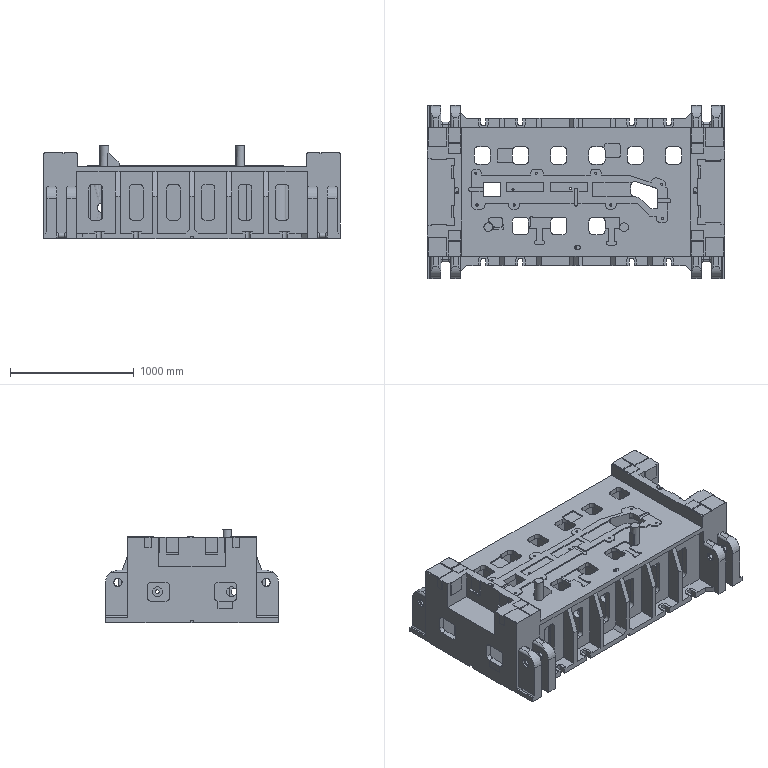Part | NX | features solid 2 | 1 solid | 1174 faces | box 2410 x 1400 x 755 mm | volume 619519304 mm3 | plane 834 | cylinder 306 | spline 26 | torus 8 | commonest cylinder face diameters 60 x97 68 x48 80 x31 40 x29 30 x27 70 x18